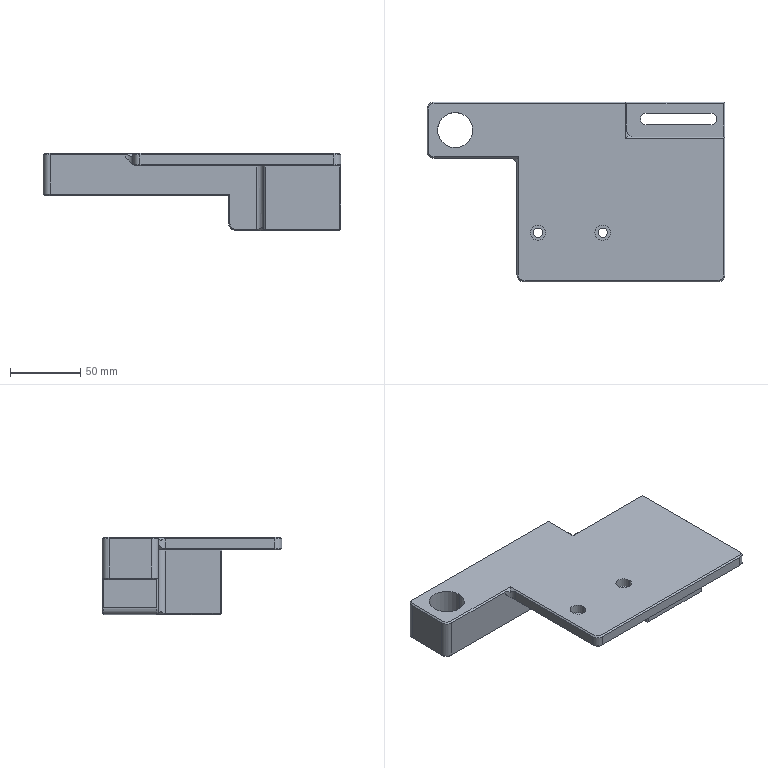NC program | NX | posted with a generic post | part box 212 x 128 x 55 mm
Lines 1 to 2819 of 8014, first 2439 of 2813 lines:
N10 G17 G21 G94 G90
(FLOOR_WALL_COPY_1 , TOOL : D50R0.8)
N12 T21 M6
N14 G54
N16 G17 G0 G90 X6.958 Y-91. S1200 M3
N18 G43 Z30. H21
N20 Z-0.45
N22 G94 G1 Y-63. F1200.
N24 X-101.
N26 G2 X-105. Y-59. R4.
N28 G1 Y-46.1
N30 X-41.603
N32 X-25.9 Y-30.397
N34 Y-1.1
N36 X41.
N38 Y-59.
N40 G2 X37. Y-63. R4.
N42 G1 X6.958
N44 Y-38.
N46 X-2.084
N48 G3 X-0.9 Y-30.397 R25.
N50 G1 Y-26.1
N52 X16.
N54 Y-38.
N56 X6.958
N58 Y-41.
N60 G0 Z30.
N62 Y-91.
N64 Z-0.9
N66 G1 Y-63.
N68 X-101.
N70 G2 X-105. Y-59. R4.
N72 G1 Y-46.1
N74 X-41.603
N76 X-25.9 Y-30.397
N78 Y-1.1
N80 X41.
N82 Y-59.
N84 G2 X37. Y-63. R4.
N86 G1 X6.958
N88 Y-38.
N90 X-2.084
N92 G3 X-0.9 Y-30.397 R25.
N94 G1 Y-26.1
N96 X16.
N98 Y-38.
N100 X6.958
N102 Y-41.
N104 G0 Z30.
N106 Y-91.
N108 Z-1.35
N110 G1 Y-63.
N112 X-101.
N114 G2 X-105. Y-59. R4.
N116 G1 Y-46.1
N118 X-41.603
N120 X-25.9 Y-30.397
N122 Y-1.1
N124 X41.
N126 Y-59.
N128 G2 X37. Y-63. R4.
N130 G1 X6.958
N132 Y-38.
N134 X-2.084
N136 G3 X-0.9 Y-30.397 R25.
N138 G1 Y-26.1
N140 X16.
N142 Y-38.
N144 X6.958
N146 Y-41.
N148 G0 Z30.
N150 Y-91.
N152 Z-1.8
N154 G1 Y-63.
N156 X-101.
N158 G2 X-105. Y-59. R4.
N160 G1 Y-46.1
N162 X-41.603
N164 X-25.9 Y-30.397
N166 Y-1.1
N168 X41.
N170 Y-59.
N172 G2 X37. Y-63. R4.
N174 G1 X6.958
N176 Y-38.
N178 X-2.084
N180 G3 X-0.9 Y-30.397 R25.
N182 G1 Y-26.1
N184 X16.
N186 Y-38.
N188 X6.958
N190 Y-41.
N192 G0 Z30.
N194 Y-91.
N196 Z-2.25
N198 G1 Y-63.
N200 X-101.
N202 G2 X-105. Y-59. R4.
N204 G1 Y-46.1
N206 X-41.603
N208 X-25.9 Y-30.397
N210 Y-1.1
N212 X41.
N214 Y-59.
N216 G2 X37. Y-63. R4.
N218 G1 X6.958
N220 Y-38.
N222 X-2.084
N224 G3 X-0.9 Y-30.397 R25.
N226 G1 Y-26.1
N228 X16.
N230 Y-38.
N232 X6.958
N234 Y-41.
N236 G0 Z30.
N238 Y-91.
N240 Z-2.7
N242 G1 Y-63.
N244 X-101.
N246 G2 X-105. Y-59. R4.
N248 G1 Y-46.1
N250 X-41.603
N252 X-25.9 Y-30.397
N254 Y-1.1
N256 X41.
N258 Y-59.
N260 G2 X37. Y-63. R4.
N262 G1 X6.958
N264 Y-38.
N266 X-2.084
N268 G3 X-0.9 Y-30.397 R25.
N270 G1 Y-26.1
N272 X16.
N274 Y-38.
N276 X6.958
N278 Y-41.
N280 G0 Z30.
N282 Y-91.
N284 Z-3.15
N286 G1 Y-63.
N288 X-101.
N290 G2 X-105. Y-59. R4.
N292 G1 Y-46.1
N294 X-41.603
N296 X-25.9 Y-30.397
N298 Y-1.1
N300 X41.
N302 Y-59.
N304 G2 X37. Y-63. R4.
N306 G1 X6.958
N308 Y-38.
N310 X-2.084
N312 G3 X-0.9 Y-30.397 R25.
N314 G1 Y-26.1
N316 X16.
N318 Y-38.
N320 X6.958
N322 Y-41.
N324 G0 Z30.
N326 Y-91.
N328 Z-3.6
N330 G1 Y-63.
N332 X-101.
N334 G2 X-105. Y-59. R4.
N336 G1 Y-46.1
N338 X-41.603
N340 X-25.9 Y-30.397
N342 Y-1.1
N344 X41.
N346 Y-59.
N348 G2 X37. Y-63. R4.
N350 G1 X6.958
N352 Y-38.
N354 X-2.084
N356 G3 X-0.9 Y-30.397 R25.
N358 G1 Y-26.1
N360 X16.
N362 Y-38.
N364 X6.958
N366 Y-41.
N368 G0 Z30.
N370 Y-91.
N372 Z-4.05
N374 G1 Y-63.
N376 X-101.
N378 G2 X-105. Y-59. R4.
N380 G1 Y-46.1
N382 X-41.603
N384 X-25.9 Y-30.397
N386 Y-1.1
N388 X41.
N390 Y-59.
N392 G2 X37. Y-63. R4.
N394 G1 X6.958
N396 Y-38.
N398 X-2.084
N400 G3 X-0.9 Y-30.397 R25.
N402 G1 Y-26.1
N404 X16.
N406 Y-38.
N408 X6.958
N410 Y-41.
N412 G0 Z30.
N414 Y-91.
N416 Z-4.5
N418 G1 Y-63.
N420 X-101.
N422 G2 X-105. Y-59. R4.
N424 G1 Y-46.1
N426 X-41.603
N428 X-25.9 Y-30.397
N430 Y-1.1
N432 X41.
N434 Y-59.
N436 G2 X37. Y-63. R4.
N438 G1 X6.958
N440 Y-38.
N442 X-2.084
N444 G3 X-0.9 Y-30.397 R25.
N446 G1 Y-26.1
N448 X16.
N450 Y-38.
N452 X6.958
N454 Y-41.
N456 G0 Z30.
N458 Y-91.
N460 Z-4.95
N462 G1 Y-63.
N464 X-101.
N466 G2 X-105. Y-59. R4.
N468 G1 Y-46.1
N470 X-41.603
N472 X-25.9 Y-30.397
N474 Y-1.1
N476 X41.
N478 Y-59.
N480 G2 X37. Y-63. R4.
N482 G1 X6.958
N484 Y-38.
N486 X-2.084
N488 G3 X-0.9 Y-30.397 R25.
N490 G1 Y-26.1
N492 X16.
N494 Y-38.
N496 X6.958
N498 Y-41.
N500 G0 Z30.
N502 Y-91.
N504 Z-5.4
N506 G1 Y-63.
N508 X-101.
N510 G2 X-105. Y-59. R4.
N512 G1 Y-46.1
N514 X-41.603
N516 X-25.9 Y-30.397
N518 Y-1.1
N520 X41.
N522 Y-59.
N524 G2 X37. Y-63. R4.
N526 G1 X6.958
N528 Y-38.
N530 X-2.084
N532 G3 X-0.9 Y-30.397 R25.
N534 G1 Y-26.1
N536 X16.
N538 Y-38.
N540 X6.958
N542 Y-41.
N544 G0 Z30.
N546 Y-91.
N548 Z-5.85
N550 G1 Y-63.
N552 X-101.
N554 G2 X-105. Y-59. R4.
N556 G1 Y-46.1
N558 X-41.603
N560 X-25.9 Y-30.397
N562 Y-1.1
N564 X41.
N566 Y-59.
N568 G2 X37. Y-63. R4.
N570 G1 X6.958
N572 Y-38.
N574 X-2.084
N576 G3 X-0.9 Y-30.397 R25.
N578 G1 Y-26.1
N580 X16.
N582 Y-38.
N584 X6.958
N586 Y-41.
N588 G0 Z30.
N590 Y-91.
N592 Z-6.3
N594 G1 Y-63.
N596 X-101.
N598 G2 X-105. Y-59. R4.
N600 G1 Y-46.1
N602 X-41.603
N604 X-25.9 Y-30.397
N606 Y-1.1
N608 X41.
N610 Y-59.
N612 G2 X37. Y-63. R4.
N614 G1 X6.958
N616 Y-38.
N618 X-2.084
N620 G3 X-0.9 Y-30.397 R25.
N622 G1 Y-26.1
N624 X16.
N626 Y-38.
N628 X6.958
N630 Y-41.
N632 G0 Z30.
N634 Y-91.
N636 Z-6.75
N638 G1 Y-63.
N640 X-101.
N642 G2 X-105. Y-59. R4.
N644 G1 Y-46.1
N646 X-41.603
N648 X-25.9 Y-30.397
N650 Y-1.1
N652 X41.
N654 Y-59.
N656 G2 X37. Y-63. R4.
N658 G1 X6.958
N660 Y-38.
N662 X-2.084
N664 G3 X-0.9 Y-30.397 R25.
N666 G1 Y-26.1
N668 X16.
N670 Y-38.
N672 X6.958
N674 Y-41.
N676 G0 Z30.
N678 Y-91.
N680 Z-7.2
N682 G1 Y-63.
N684 X-101.
N686 G2 X-105. Y-59. R4.
N688 G1 Y-46.1
N690 X-41.603
N692 X-25.9 Y-30.397
N694 Y-1.1
N696 X41.
N698 Y-59.
N700 G2 X37. Y-63. R4.
N702 G1 X6.958
N704 Y-38.
N706 X-2.084
N708 G3 X-0.9 Y-30.397 R25.
N710 G1 Y-26.1
N712 X16.
N714 Y-38.
N716 X6.958
N718 Y-41.
N720 G0 Z30.
N722 Y-91.
N724 Z-7.65
N726 G1 Y-63.
N728 X-101.
N730 G2 X-105. Y-59. R4.
N732 G1 Y-46.1
N734 X-41.603
N736 X-25.9 Y-30.397
N738 Y-1.1
N740 X41.
N742 Y-59.
N744 G2 X37. Y-63. R4.
N746 G1 X6.958
N748 Y-38.
N750 X-2.084
N752 G3 X-0.9 Y-30.397 R25.
N754 G1 Y-26.1
N756 X16.
N758 Y-38.
N760 X6.958
N762 Y-41.
N764 G0 Z30.
N766 Y-91.
N768 Z-8.1
N770 G1 Y-63.
N772 X-101.
N774 G2 X-105. Y-59. R4.
N776 G1 Y-46.1
N778 X-41.603
N780 X-25.9 Y-30.397
N782 Y-1.1
N784 X41.
N786 Y-59.
N788 G2 X37. Y-63. R4.
N790 G1 X6.958
N792 Y-38.
N794 X-2.084
N796 G3 X-0.9 Y-30.397 R25.
N798 G1 Y-26.1
N800 X16.
N802 Y-38.
N804 X6.958
N806 Y-41.
N808 G0 Z30.
N810 Y-91.
N812 Z-8.55
N814 G1 Y-63.
N816 X-101.
N818 G2 X-105. Y-59. R4.
N820 G1 Y-46.1
N822 X-41.603
N824 X-25.9 Y-30.397
N826 Y-1.1
N828 X41.
N830 Y-59.
N832 G2 X37. Y-63. R4.
N834 G1 X6.958
N836 Y-38.
N838 X-2.084
N840 G3 X-0.9 Y-30.397 R25.
N842 G1 Y-26.1
N844 X16.
N846 Y-38.
N848 X6.958
N850 Y-41.
N852 G0 Z30.
N854 Y-91.
N856 Z-9.
N858 G1 Y-63.
N860 X-101.
N862 G2 X-105. Y-59. R4.
N864 G1 Y-46.1
N866 X-41.603
N868 X-25.9 Y-30.397
N870 Y-1.1
N872 X41.
N874 Y-59.
N876 G2 X37. Y-63. R4.
N878 G1 X6.958
N880 Y-38.
N882 X-2.084
N884 G3 X-0.9 Y-30.397 R25.
N886 G1 Y-26.1
N888 X16.
N890 Y-38.
N892 X6.958
N894 Y-41.
N896 G0 Z30.
N898 Y-91.
N900 Z-9.45
N902 G1 Y-63.
N904 X-101.
N906 G2 X-105. Y-59. R4.
N908 G1 Y-46.1
N910 X-41.603
N912 X-25.9 Y-30.397
N914 Y-1.1
N916 X41.
N918 Y-59.
N920 G2 X37. Y-63. R4.
N922 G1 X6.958
N924 Y-38.
N926 X-2.084
N928 G3 X-0.9 Y-30.397 R25.
N930 G1 Y-26.1
N932 X16.
N934 Y-38.
N936 X6.958
N938 Y-41.
N940 G0 Z30.
N942 Y-91.
N944 Z-9.9
N946 G1 Y-63.
N948 X-101.
N950 G2 X-105. Y-59. R4.
N952 G1 Y-46.1
N954 X-41.603
N956 X-25.9 Y-30.397
N958 Y-1.1
N960 X41.
N962 Y-59.
N964 G2 X37. Y-63. R4.
N966 G1 X6.958
N968 Y-38.
N970 X-2.084
N972 G3 X-0.9 Y-30.397 R25.
N974 G1 Y-26.1
N976 X16.
N978 Y-38.
N980 X6.958
N982 Y-41.
N984 G0 Z30.
N986 Y-91.
N988 Z-10.35
N990 G1 Y-63.
N992 X-101.
N994 G2 X-105. Y-59. R4.
N996 G1 Y-46.1
N998 X-41.603
N1000 X-25.9 Y-30.397
N1002 Y-1.1
N1004 X41.
N1006 Y-59.
N1008 G2 X37. Y-63. R4.
N1010 G1 X6.958
N1012 Y-38.
N1014 X-2.084
N1016 G3 X-0.9 Y-30.397 R25.
N1018 G1 Y-26.1
N1020 X16.
N1022 Y-38.
N1024 X6.958
N1026 Y-41.
N1028 G0 Z30.
N1030 Y-91.
N1032 Z-10.8
N1034 G1 Y-63.
N1036 X-101.
N1038 G2 X-105. Y-59. R4.
N1040 G1 Y-46.1
N1042 X-41.603
N1044 X-25.9 Y-30.397
N1046 Y-1.1
N1048 X41.
N1050 Y-59.
N1052 G2 X37. Y-63. R4.
N1054 G1 X6.958
N1056 Y-38.
N1058 X-2.084
N1060 G3 X-0.9 Y-30.397 R25.
N1062 G1 Y-26.1
N1064 X16.
N1066 Y-38.
N1068 X6.958
N1070 Y-41.
N1072 G0 Z30.
N1074 Y-91.
N1076 Z-11.25
N1078 G1 Y-63.
N1080 X-101.
N1082 G2 X-105. Y-59. R4.
N1084 G1 Y-46.1
N1086 X-41.603
N1088 X-25.9 Y-30.397
N1090 Y-1.1
N1092 X41.
N1094 Y-59.
N1096 G2 X37. Y-63. R4.
N1098 G1 X6.958
N1100 Y-38.
N1102 X-2.084
N1104 G3 X-0.9 Y-30.397 R25.
N1106 G1 Y-26.1
N1108 X16.
N1110 Y-38.
N1112 X6.958
N1114 Y-41.
N1116 G0 Z30.
N1118 Y-91.
N1120 Z-11.7
N1122 G1 Y-63.
N1124 X-101.
N1126 G2 X-105. Y-59. R4.
N1128 G1 Y-46.1
N1130 X-41.603
N1132 X-25.9 Y-30.397
N1134 Y-1.1
N1136 X41.
N1138 Y-59.
N1140 G2 X37. Y-63. R4.
N1142 G1 X6.958
N1144 Y-38.
N1146 X-2.084
N1148 G3 X-0.9 Y-30.397 R25.
N1150 G1 Y-26.1
N1152 X16.
N1154 Y-38.
N1156 X6.958
N1158 Y-41.
N1160 G0 Z30.
N1162 Y-91.
N1164 Z-12.15
N1166 G1 Y-63.
N1168 X-101.
N1170 G2 X-105. Y-59. R4.
N1172 G1 Y-46.1
N1174 X-41.603
N1176 X-25.9 Y-30.397
N1178 Y-1.1
N1180 X41.
N1182 Y-59.
N1184 G2 X37. Y-63. R4.
N1186 G1 X6.958
N1188 Y-38.
N1190 X-2.084
N1192 G3 X-0.9 Y-30.397 R25.
N1194 G1 Y-26.1
N1196 X16.
N1198 Y-38.
N1200 X6.958
N1202 Y-41.
N1204 G0 Z30.
N1206 Y-91.
N1208 Z-12.6
N1210 G1 Y-63.
N1212 X-101.
N1214 G2 X-105. Y-59. R4.
N1216 G1 Y-46.1
N1218 X-41.603
N1220 X-25.9 Y-30.397
N1222 Y-1.1
N1224 X41.
N1226 Y-59.
N1228 G2 X37. Y-63. R4.
N1230 G1 X6.958
N1232 Y-38.
N1234 X-2.084
N1236 G3 X-0.9 Y-30.397 R25.
N1238 G1 Y-26.1
N1240 X16.
N1242 Y-38.
N1244 X6.958
N1246 Y-41.
N1248 G0 Z30.
N1250 Y-91.
N1252 Z-13.05
N1254 G1 Y-63.
N1256 X-101.
N1258 G2 X-105. Y-59. R4.
N1260 G1 Y-46.1
N1262 X-41.603
N1264 X-25.9 Y-30.397
N1266 Y-1.1
N1268 X41.
N1270 Y-59.
N1272 G2 X37. Y-63. R4.
N1274 G1 X6.958
N1276 Y-38.
N1278 X-2.084
N1280 G3 X-0.9 Y-30.397 R25.
N1282 G1 Y-26.1
N1284 X16.
N1286 Y-38.
N1288 X6.958
N1290 Y-41.
N1292 G0 Z30.
N1294 Y-91.
N1296 Z-13.5
N1298 G1 Y-63.
N1300 X-101.
N1302 G2 X-105. Y-59. R4.
N1304 G1 Y-46.1
N1306 X-41.603
N1308 X-25.9 Y-30.397
N1310 Y-1.1
N1312 X41.
N1314 Y-59.
N1316 G2 X37. Y-63. R4.
N1318 G1 X6.958
N1320 Y-38.
N1322 X-2.084
N1324 G3 X-0.9 Y-30.397 R25.
N1326 G1 Y-26.1
N1328 X16.
N1330 Y-38.
N1332 X6.958
N1334 Y-41.
N1336 G0 Z30.
N1338 Y-91.
N1340 Z-13.95
N1342 G1 Y-63.
N1344 X-101.
N1346 G2 X-105. Y-59. R4.
N1348 G1 Y-46.1
N1350 X-41.603
N1352 X-25.9 Y-30.397
N1354 Y-1.1
N1356 X41.
N1358 Y-59.
N1360 G2 X37. Y-63. R4.
N1362 G1 X6.958
N1364 Y-38.
N1366 X-2.084
N1368 G3 X-0.9 Y-30.397 R25.
N1370 G1 Y-26.1
N1372 X16.
N1374 Y-38.
N1376 X6.958
N1378 Y-41.
N1380 G0 Z30.
N1382 Y-91.
N1384 Z-14.4
N1386 G1 Y-63.
N1388 X-101.
N1390 G2 X-105. Y-59. R4.
N1392 G1 Y-46.1
N1394 X-41.603
N1396 X-25.9 Y-30.397
N1398 Y-1.1
N1400 X41.
N1402 Y-59.
N1404 G2 X37. Y-63. R4.
N1406 G1 X6.958
N1408 Y-38.
N1410 X-2.084
N1412 G3 X-0.9 Y-30.397 R25.
N1414 G1 Y-26.1
N1416 X16.
N1418 Y-38.
N1420 X6.958
N1422 Y-41.
N1424 G0 Z30.
N1426 Y-91.
N1428 Z-14.85
N1430 G1 Y-63.
N1432 X-101.
N1434 G2 X-105. Y-59. R4.
N1436 G1 Y-46.1
N1438 X-41.603
N1440 X-25.9 Y-30.397
N1442 Y-1.1
N1444 X41.
N1446 Y-59.
N1448 G2 X37. Y-63. R4.
N1450 G1 X6.958
N1452 Y-38.
N1454 X-2.084
N1456 G3 X-0.9 Y-30.397 R25.
N1458 G1 Y-26.1
N1460 X16.
N1462 Y-38.
N1464 X6.958
N1466 Y-41.
N1468 G0 Z30.
N1470 Y-91.
N1472 Z-15.3
N1474 G1 Y-63.
N1476 X-101.
N1478 G2 X-105. Y-59. R4.
N1480 G1 Y-46.1
N1482 X-41.603
N1484 X-25.9 Y-30.397
N1486 Y-1.1
N1488 X41.
N1490 Y-59.
N1492 G2 X37. Y-63. R4.
N1494 G1 X6.958
N1496 Y-38.
N1498 X-2.084
N1500 G3 X-0.9 Y-30.397 R25.
N1502 G1 Y-26.1
N1504 X16.
N1506 Y-38.
N1508 X6.958
N1510 Y-41.
N1512 G0 Z30.
N1514 Y-91.
N1516 Z-15.75
N1518 G1 Y-63.
N1520 X-101.
N1522 G2 X-105. Y-59. R4.
N1524 G1 Y-46.1
N1526 X-41.603
N1528 X-25.9 Y-30.397
N1530 Y-1.1
N1532 X41.
N1534 Y-59.
N1536 G2 X37. Y-63. R4.
N1538 G1 X6.958
N1540 Y-38.
N1542 X-2.084
N1544 G3 X-0.9 Y-30.397 R25.
N1546 G1 Y-26.1
N1548 X16.
N1550 Y-38.
N1552 X6.958
N1554 Y-41.
N1556 G0 Z30.
N1558 Y-91.
N1560 Z-16.2
N1562 G1 Y-63.
N1564 X-101.
N1566 G2 X-105. Y-59. R4.
N1568 G1 Y-46.1
N1570 X-41.603
N1572 X-25.9 Y-30.397
N1574 Y-1.1
N1576 X41.
N1578 Y-59.
N1580 G2 X37. Y-63. R4.
N1582 G1 X6.958
N1584 Y-38.
N1586 X-2.084
N1588 G3 X-0.9 Y-30.397 R25.
N1590 G1 Y-26.1
N1592 X16.
N1594 Y-38.
N1596 X6.958
N1598 Y-41.
N1600 G0 Z30.
N1602 Y-91.
N1604 Z-16.65
N1606 G1 Y-63.
N1608 X-101.
N1610 G2 X-105. Y-59. R4.
N1612 G1 Y-46.1
N1614 X-41.603
N1616 X-25.9 Y-30.397
N1618 Y-1.1
N1620 X41.
N1622 Y-59.
N1624 G2 X37. Y-63. R4.
N1626 G1 X6.958
N1628 Y-38.
N1630 X-2.084
N1632 G3 X-0.9 Y-30.397 R25.
N1634 G1 Y-26.1
N1636 X16.
N1638 Y-38.
N1640 X6.958
N1642 Y-41.
N1644 G0 Z30.
N1646 Y-91.
N1648 Z-17.1
N1650 G1 Y-63.
N1652 X-101.
N1654 G2 X-105. Y-59. R4.
N1656 G1 Y-46.1
N1658 X-41.603
N1660 X-25.9 Y-30.397
N1662 Y-1.1
N1664 X41.
N1666 Y-59.
N1668 G2 X37. Y-63. R4.
N1670 G1 X6.958
N1672 Y-38.
N1674 X-2.084
N1676 G3 X-0.9 Y-30.397 R25.
N1678 G1 Y-26.1
N1680 X16.
N1682 Y-38.
N1684 X6.958
N1686 Y-41.
N1688 G0 Z30.
N1690 Y-91.
N1692 Z-17.55
N1694 G1 Y-63.
N1696 X-101.
N1698 G2 X-105. Y-59. R4.
N1700 G1 Y-46.1
N1702 X-41.603
N1704 X-25.9 Y-30.397
N1706 Y-1.1
N1708 X41.
N1710 Y-59.
N1712 G2 X37. Y-63. R4.
N1714 G1 X6.958
N1716 Y-38.
N1718 X-2.084
N1720 G3 X-0.9 Y-30.397 R25.
N1722 G1 Y-26.1
N1724 X16.
N1726 Y-38.
N1728 X6.958
N1730 Y-41.
N1732 G0 Z30.
N1734 Y-91.
N1736 Z-18.
N1738 G1 Y-63.
N1740 X-101.
N1742 G2 X-105. Y-59. R4.
N1744 G1 Y-46.1
N1746 X-41.603
N1748 X-25.9 Y-30.397
N1750 Y-1.1
N1752 X41.
N1754 Y-59.
N1756 G2 X37. Y-63. R4.
N1758 G1 X6.958
N1760 Y-38.
N1762 X-2.084
N1764 G3 X-0.9 Y-30.397 R25.
N1766 G1 Y-26.1
N1768 X16.
N1770 Y-38.
N1772 X6.958
N1774 Y-41.
N1776 G0 Z30.
N1778 Y-91.
N1780 Z-18.45
N1782 G1 Y-63.
N1784 X-101.
N1786 G2 X-105. Y-59. R4.
N1788 G1 Y-46.1
N1790 X-41.603
N1792 X-25.9 Y-30.397
N1794 Y-1.1
N1796 X41.
N1798 Y-59.
N1800 G2 X37. Y-63. R4.
N1802 G1 X6.958
N1804 Y-38.
N1806 X-2.084
N1808 G3 X-0.9 Y-30.397 R25.
N1810 G1 Y-26.1
N1812 X16.
N1814 Y-38.
N1816 X6.958
N1818 Y-41.
N1820 G0 Z30.
N1822 Y-91.
N1824 Z-18.9
N1826 G1 Y-63.
N1828 X-101.
N1830 G2 X-105. Y-59. R4.
N1832 G1 Y-46.1
N1834 X-41.603
N1836 X-25.9 Y-30.397
N1838 Y-1.1
N1840 X41.
N1842 Y-59.
N1844 G2 X37. Y-63. R4.
N1846 G1 X6.958
N1848 Y-38.
N1850 X-2.084
N1852 G3 X-0.9 Y-30.397 R25.
N1854 G1 Y-26.1
N1856 X16.
N1858 Y-38.
N1860 X6.958
N1862 Y-41.
N1864 G0 Z30.
N1866 Y-91.
N1868 Z-19.35
N1870 G1 Y-63.
N1872 X-101.
N1874 G2 X-105. Y-59. R4.
N1876 G1 Y-46.1
N1878 X-41.603
N1880 X-25.9 Y-30.397
N1882 Y-1.1
N1884 X41.
N1886 Y-59.
N1888 G2 X37. Y-63. R4.
N1890 G1 X6.958
N1892 Y-38.
N1894 X-2.084
N1896 G3 X-0.9 Y-30.397 R25.
N1898 G1 Y-26.1
N1900 X16.
N1902 Y-38.
N1904 X6.958
N1906 Y-41.
N1908 G0 Z30.
N1910 Y-91.
N1912 Z-19.8
N1914 G1 Y-63.
N1916 X-101.
N1918 G2 X-105. Y-59. R4.
N1920 G1 Y-46.1
N1922 X-41.603
N1924 X-25.9 Y-30.397
N1926 Y-1.1
N1928 X41.
N1930 Y-59.
N1932 G2 X37. Y-63. R4.
N1934 G1 X6.958
N1936 Y-38.
N1938 X-2.084
N1940 G3 X-0.9 Y-30.397 R25.
N1942 G1 Y-26.1
N1944 X16.
N1946 Y-38.
N1948 X6.958
N1950 Y-41.
N1952 G0 Z30.
N1954 Y-91.
N1956 Z-20.25
N1958 G1 Y-63.
N1960 X-101.
N1962 G2 X-105. Y-59. R4.
N1964 G1 Y-46.1
N1966 X-41.603
N1968 X-25.9 Y-30.397
N1970 Y-1.1
N1972 X41.
N1974 Y-59.
N1976 G2 X37. Y-63. R4.
N1978 G1 X6.958
N1980 Y-38.
N1982 X-2.084
N1984 G3 X-0.9 Y-30.397 R25.
N1986 G1 Y-26.1
N1988 X16.
N1990 Y-38.
N1992 X6.958
N1994 Y-41.
N1996 G0 Z30.
N1998 Y-91.
N2000 Z-20.7
N2002 G1 Y-63.
N2004 X-101.
N2006 G2 X-105. Y-59. R4.
N2008 G1 Y-46.1
N2010 X-41.603
N2012 X-25.9 Y-30.397
N2014 Y-1.1
N2016 X41.
N2018 Y-59.
N2020 G2 X37. Y-63. R4.
N2022 G1 X6.958
N2024 Y-38.
N2026 X-2.084
N2028 G3 X-0.9 Y-30.397 R25.
N2030 G1 Y-26.1
N2032 X16.
N2034 Y-38.
N2036 X6.958
N2038 Y-41.
N2040 G0 Z30.
N2042 Y-91.
N2044 Z-21.15
N2046 G1 Y-63.
N2048 X-101.
N2050 G2 X-105. Y-59. R4.
N2052 G1 Y-46.1
N2054 X-41.603
N2056 X-25.9 Y-30.397
N2058 Y-1.1
N2060 X41.
N2062 Y-59.
N2064 G2 X37. Y-63. R4.
N2066 G1 X6.958
N2068 Y-38.
N2070 X-2.084
N2072 G3 X-0.9 Y-30.397 R25.
N2074 G1 Y-26.1
N2076 X16.
N2078 Y-38.
N2080 X6.958
N2082 Y-41.
N2084 G0 Z30.
N2086 Y-91.
N2088 Z-21.6
N2090 G1 Y-63.
N2092 X-101.
N2094 G2 X-105. Y-59. R4.
N2096 G1 Y-46.1
N2098 X-41.603
N2100 X-25.9 Y-30.397
N2102 Y-1.1
N2104 X41.
N2106 Y-59.
N2108 G2 X37. Y-63. R4.
N2110 G1 X6.958
N2112 Y-38.
N2114 X-2.084
N2116 G3 X-0.9 Y-30.397 R25.
N2118 G1 Y-26.1
N2120 X16.
N2122 Y-38.
N2124 X6.958
N2126 Y-41.
N2128 G0 Z30.
N2130 Y-91.
N2132 Z-22.05
N2134 G1 Y-63.
N2136 X-101.
N2138 G2 X-105. Y-59. R4.
N2140 G1 Y-46.1
N2142 X-41.603
N2144 X-25.9 Y-30.397
N2146 Y-1.1
N2148 X41.
N2150 Y-59.
N2152 G2 X37. Y-63. R4.
N2154 G1 X6.958
N2156 Y-38.
N2158 X-2.084
N2160 G3 X-0.9 Y-30.397 R25.
N2162 G1 Y-26.1
N2164 X16.
N2166 Y-38.
N2168 X6.958
N2170 Y-41.
N2172 G0 Z30.
N2174 Y-91.
N2176 Z-22.5
N2178 G1 Y-63.
N2180 X-101.
N2182 G2 X-105. Y-59. R4.
N2184 G1 Y-46.1
N2186 X-41.603
N2188 X-25.9 Y-30.397
N2190 Y-1.1
N2192 X41.
N2194 Y-59.
N2196 G2 X37. Y-63. R4.
N2198 G1 X6.958
N2200 Y-38.
N2202 X-2.084
N2204 G3 X-0.9 Y-30.397 R25.
N2206 G1 Y-26.1
N2208 X16.
N2210 Y-38.
N2212 X6.958
N2214 Y-41.
N2216 G0 Z30.
N2218 Y-91.
N2220 Z-22.95
N2222 G1 Y-63.
N2224 X-101.
N2226 G2 X-105. Y-59. R4.
N2228 G1 Y-46.1
N2230 X-41.603
N2232 X-25.9 Y-30.397
N2234 Y-1.1
N2236 X41.
N2238 Y-59.
N2240 G2 X37. Y-63. R4.
N2242 G1 X6.958
N2244 Y-38.
N2246 X-2.084
N2248 G3 X-0.9 Y-30.397 R25.
N2250 G1 Y-26.1
N2252 X16.
N2254 Y-38.
N2256 X6.958
N2258 Y-41.
N2260 G0 Z30.
N2262 Y-91.
N2264 Z-23.4
N2266 G1 Y-63.
N2268 X-101.
N2270 G2 X-105. Y-59. R4.
N2272 G1 Y-46.1
N2274 X-41.603
N2276 X-25.9 Y-30.397
N2278 Y-1.1
N2280 X41.
N2282 Y-59.
N2284 G2 X37. Y-63. R4.
N2286 G1 X6.958
N2288 Y-38.
N2290 X-2.084
N2292 G3 X-0.9 Y-30.397 R25.
N2294 G1 Y-26.1
N2296 X16.
N2298 Y-38.
N2300 X6.958
N2302 Y-41.
N2304 G0 Z30.
N2306 Y-91.
N2308 Z-23.85
N2310 G1 Y-63.
N2312 X-101.
N2314 G2 X-105. Y-59. R4.
N2316 G1 Y-46.1
N2318 X-41.603
N2320 X-25.9 Y-30.397
N2322 Y-1.1
N2324 X41.
N2326 Y-59.
N2328 G2 X37. Y-63. R4.
N2330 G1 X6.958
N2332 Y-38.
N2334 X-2.084
N2336 G3 X-0.9 Y-30.397 R25.
N2338 G1 Y-26.1
N2340 X16.
N2342 Y-38.
N2344 X6.958
N2346 Y-41.
N2348 G0 Z30.
N2350 Y-91.
N2352 Z-24.3
N2354 G1 Y-63.
N2356 X-101.
N2358 G2 X-105. Y-59. R4.
N2360 G1 Y-46.1
N2362 X-41.603
N2364 X-25.9 Y-30.397
N2366 Y-1.1
N2368 X41.
N2370 Y-59.
N2372 G2 X37. Y-63. R4.
N2374 G1 X6.958
N2376 Y-38.
N2378 X-2.084
N2380 G3 X-0.9 Y-30.397 R25.
N2382 G1 Y-26.1
N2384 X16.
N2386 Y-38.
N2388 X6.958
N2390 Y-41.
N2392 G0 Z30.
N2394 Y-91.
N2396 Z-24.75
N2398 G1 Y-63.
N2400 X-101.
N2402 G2 X-105. Y-59. R4.
N2404 G1 Y-46.1
N2406 X-41.603
N2408 X-25.9 Y-30.397
N2410 Y-1.1
N2412 X41.
N2414 Y-59.
N2416 G2 X37. Y-63. R4.
N2418 G1 X6.958
N2420 Y-38.
N2422 X-2.084
N2424 G3 X-0.9 Y-30.397 R25.
N2426 G1 Y-26.1
N2428 X16.
N2430 Y-38.
N2432 X6.958
N2434 Y-41.
N2436 G0 Z30.
N2438 Y-91.
N2440 Z-25.2
N2442 G1 Y-63.
N2444 X-101.
N2446 G2 X-105. Y-59. R4.
N2448 G1 Y-46.1
N2450 X-41.603
N2452 X-25.9 Y-30.397
N2454 Y-1.1
N2456 X41.
N2458 Y-59.
N2460 G2 X37. Y-63. R4.
N2462 G1 X6.958
N2464 Y-38.
N2466 X-2.084
N2468 G3 X-0.9 Y-30.397 R25.
N2470 G1 Y-26.1
N2472 X16.
N2474 Y-38.
N2476 X6.958
N2478 Y-41.
N2480 G0 Z30.
N2482 Y-91.
N2484 Z-25.65
N2486 G1 Y-63.
N2488 X-101.
N2490 G2 X-105. Y-59. R4.
N2492 G1 Y-46.1
N2494 X-41.603
N2496 X-25.9 Y-30.397
N2498 Y-1.1
N2500 X41.
N2502 Y-59.
N2504 G2 X37. Y-63. R4.
N2506 G1 X6.958
N2508 Y-38.
N2510 X-2.084
N2512 G3 X-0.9 Y-30.397 R25.
N2514 G1 Y-26.1
N2516 X16.
N2518 Y-38.
N2520 X6.958
N2522 Y-41.
N2524 G0 Z30.
N2526 Y-91.
N2528 Z-26.1
N2530 G1 Y-63.
N2532 X-101.
N2534 G2 X-105. Y-59. R4.
N2536 G1 Y-46.1
N2538 X-41.603
N2540 X-25.9 Y-30.397
N2542 Y-1.1
N2544 X41.
N2546 Y-59.
N2548 G2 X37. Y-63. R4.
N2550 G1 X6.958
N2552 Y-38.
N2554 X-2.084
N2556 G3 X-0.9 Y-30.397 R25.
N2558 G1 Y-26.1
N2560 X16.
N2562 Y-38.
N2564 X6.958
N2566 Y-41.
N2568 G0 Z30.
N2570 Y-91.
N2572 Z-26.55
N2574 G1 Y-63.
N2576 X-101.
N2578 G2 X-105. Y-59. R4.
N2580 G1 Y-46.1
N2582 X-41.603
N2584 X-25.9 Y-30.397
N2586 Y-1.1
N2588 X41.
N2590 Y-59.
N2592 G2 X37. Y-63. R4.
N2594 G1 X6.958
N2596 Y-38.
N2598 X-2.084
N2600 G3 X-0.9 Y-30.397 R25.
N2602 G1 Y-26.1
N2604 X16.
N2606 Y-38.
N2608 X6.958
N2610 Y-41.
N2612 G0 Z30.
N2614 Y-91.
N2616 Z-27.
N2618 G1 Y-63.
N2620 X-101.
N2622 G2 X-105. Y-59. R4.
N2624 G1 Y-46.1
N2626 X-41.603
N2628 X-25.9 Y-30.397
N2630 Y-1.1
N2632 X41.
N2634 Y-59.
N2636 G2 X37. Y-63. R4.
N2638 G1 X6.958
N2640 Y-38.
N2642 X-2.084
N2644 G3 X-0.9 Y-30.397 R25.
N2646 G1 Y-26.1
N2648 X16.
N2650 Y-38.
N2652 X6.958
N2654 Y-41.
N2656 G0 Z30.
N2658 Y-91.
N2660 Z-27.45
N2662 G1 Y-63.
N2664 X-101.
N2666 G2 X-105. Y-59. R4.
N2668 G1 Y-46.1
N2670 X-41.603
N2672 X-25.9 Y-30.397
N2674 Y-1.1
N2676 X41.
N2678 Y-59.
N2680 G2 X37. Y-63. R4.
N2682 G1 X6.958
N2684 Y-38.
N2686 X-2.084
N2688 G3 X-0.9 Y-30.397 R25.
N2690 G1 Y-26.1
N2692 X16.
N2694 Y-38.
N2696 X6.958
N2698 Y-41.
N2700 G0 Z30.
N2702 Y-91.
N2704 Z-27.9
N2706 G1 Y-63.
N2708 X-101.
N2710 G2 X-105. Y-59. R4.
N2712 G1 Y-46.1
N2714 X-41.603
N2716 X-25.9 Y-30.397
N2718 Y-1.1
N2720 X41.
N2722 Y-59.
N2724 G2 X37. Y-63. R4.
N2726 G1 X6.958
N2728 Y-38.
N2730 X-2.084
N2732 G3 X-0.9 Y-30.397 R25.
N2734 G1 Y-26.1
N2736 X16.
N2738 Y-38.
N2740 X6.958
N2742 Y-41.
N2744 G0 Z30.
N2746 Y-91.
N2748 Z-28.35
N2750 G1 Y-63.
N2752 X-101.
N2754 G2 X-105. Y-59. R4.
N2756 G1 Y-46.1
N2758 X-41.603
N2760 X-25.9 Y-30.397
N2762 Y-1.1
N2764 X41.
N2766 Y-59.
N2768 G2 X37. Y-63. R4.
N2770 G1 X6.958
N2772 Y-38.
N2774 X-2.084
N2776 G3 X-0.9 Y-30.397 R25.
N2778 G1 Y-26.1
N2780 X16.
N2782 Y-38.
N2784 X6.958
N2786 Y-41.
N2788 G0 Z30.
N2790 Y-91.
N2792 Z-28.8
N2794 G1 Y-63.
N2796 X-101.
N2798 G2 X-105. Y-59. R4.
N2800 G1 Y-46.1
N2802 X-41.603
N2804 X-25.9 Y-30.397
N2806 Y-1.1
N2808 X41.
N2810 Y-59.
N2812 G2 X37. Y-63. R4.
N2814 G1 X6.958
N2816 Y-38.
N2818 X-2.084
N2820 G3 X-0.9 Y-30.397 R25.
N2822 G1 Y-26.1
N2824 X16.
N2826 Y-38.
N2828 X6.958
N2830 Y-41.
N2832 G0 Z30.
N2834 Y-91.
N2836 Z-29.25
N2838 G1 Y-63.
N2840 X-101.
N2842 G2 X-105. Y-59. R4.
N2844 G1 Y-46.1
N2846 X-41.603
N2848 X-25.9 Y-30.397
N2850 Y-1.1
N2852 X41.
N2854 Y-59.
N2856 G2 X37. Y-63. R4.
N2858 G1 X6.958
N2860 Y-38.
N2862 X-2.084
N2864 G3 X-0.9 Y-30.397 R25.
N2866 G1 Y-26.1
N2868 X16.
N2870 Y-38.
N2872 X6.958
N2874 Y-41.
N2876 G0 Z30.
N2878 Y-91.
N2880 Z-29.7
N2882 G1 Y-63.
N2884 X-101.
N2886 G2 X-105. Y-59. R4.
N2888 G1 Y-46.1
N2890 X-41.603
N2892 X-25.9 Y-30.397
N2894 Y-1.1
N2896 X41.
N2898 Y-59.
N2900 G2 X37. Y-63. R4.
N2902 G1 X6.958
N2904 Y-38.
N2906 X-2.084
N2908 G3 X-0.9 Y-30.397 R25.
N2910 G1 Y-26.1
N2912 X16.
N2914 Y-38.
N2916 X6.958
N2918 Y-41.
N2920 G0 Z30.
N2922 Y-91.
N2924 Z-30.15
N2926 G1 Y-63.
N2928 X-101.
N2930 G2 X-105. Y-59. R4.
N2932 G1 Y-46.1
N2934 X-41.603
N2936 X-25.9 Y-30.397
N2938 Y-1.1
N2940 X41.
N2942 Y-59.
N2944 G2 X37. Y-63. R4.
N2946 G1 X6.958
N2948 Y-38.
N2950 X-2.084
N2952 G3 X-0.9 Y-30.397 R25.
N2954 G1 Y-26.1
N2956 X16.
N2958 Y-38.
N2960 X6.958
N2962 Y-41.
N2964 G0 Z30.
N2966 Y-91.
N2968 Z-30.6
N2970 G1 Y-63.
N2972 X-101.
N2974 G2 X-105. Y-59. R4.
N2976 G1 Y-46.1
N2978 X-41.603
N2980 X-25.9 Y-30.397
N2982 Y-1.1
N2984 X41.
N2986 Y-59.
N2988 G2 X37. Y-63. R4.
N2990 G1 X6.958
N2992 Y-38.
N2994 X-2.084
N2996 G3 X-0.9 Y-30.397 R25.
N2998 G1 Y-26.1
N3000 X16.
N3002 Y-38.
N3004 X6.958
N3006 Y-41.
N3008 G0 Z30.
N3010 Y-91.
N3012 Z-31.05
N3014 G1 Y-63.
N3016 X-101.
N3018 G2 X-105. Y-59. R4.
N3020 G1 Y-46.1
N3022 X-41.603
N3024 X-25.9 Y-30.397
N3026 Y-1.1
N3028 X41.
N3030 Y-59.
N3032 G2 X37. Y-63. R4.
N3034 G1 X6.958
N3036 Y-38.
N3038 X-2.084
N3040 G3 X-0.9 Y-30.397 R25.
N3042 G1 Y-26.1
N3044 X16.
N3046 Y-38.
N3048 X6.958
N3050 Y-41.
N3052 G0 Z30.
N3054 Y-91.
N3056 Z-31.5
N3058 G1 Y-63.
N3060 X-101.
N3062 G2 X-105. Y-59. R4.
N3064 G1 Y-46.1
N3066 X-41.603
N3068 X-25.9 Y-30.397
N3070 Y-1.1
N3072 X41.
N3074 Y-59.
N3076 G2 X37. Y-63. R4.
N3078 G1 X6.958
N3080 Y-38.
N3082 X-2.084
N3084 G3 X-0.9 Y-30.397 R25.
N3086 G1 Y-26.1
N3088 X16.
N3090 Y-38.
N3092 X6.958
N3094 Y-41.
N3096 G0 Z30.
N3098 Y-91.
N3100 Z-31.95
N3102 G1 Y-63.
N3104 X-101.
N3106 G2 X-105. Y-59. R4.
N3108 G1 Y-46.1
N3110 X-41.603
N3112 X-25.9 Y-30.397
N3114 Y-1.1
N3116 X41.
N3118 Y-59.
N3120 G2 X37. Y-63. R4.
N3122 G1 X6.958
N3124 Y-38.
N3126 X-2.084
N3128 G3 X-0.9 Y-30.397 R25.
N3130 G1 Y-26.1
N3132 X16.
N3134 Y-38.
N3136 X6.958
N3138 Y-41.
N3140 G0 Z30.
N3142 Y-91.
N3144 Z-32.4
N3146 G1 Y-63.
N3148 X-101.
N3150 G2 X-105. Y-59. R4.
N3152 G1 Y-46.1
N3154 X-41.603
N3156 X-25.9 Y-30.397
N3158 Y-1.1
N3160 X41.
N3162 Y-59.
N3164 G2 X37. Y-63. R4.
N3166 G1 X6.958
N3168 Y-38.
N3170 X-2.084
N3172 G3 X-0.9 Y-30.397 R25.
N3174 G1 Y-26.1
N3176 X16.
N3178 Y-38.
N3180 X6.958
N3182 Y-41.
N3184 G0 Z30.
N3186 Y-91.
N3188 Z-32.85
N3190 G1 Y-63.
N3192 X-101.
N3194 G2 X-105. Y-59. R4.
N3196 G1 Y-46.1
N3198 X-41.603
N3200 X-25.9 Y-30.397
N3202 Y-1.1
N3204 X41.
N3206 Y-59.
N3208 G2 X37. Y-63. R4.
N3210 G1 X6.958
N3212 Y-38.
N3214 X-2.084
N3216 G3 X-0.9 Y-30.397 R25.
N3218 G1 Y-26.1
N3220 X16.
N3222 Y-38.
N3224 X6.958
N3226 Y-41.
N3228 G0 Z30.
N3230 Y-91.
N3232 Z-33.3
N3234 G1 Y-63.
N3236 X-101.
N3238 G2 X-105. Y-59. R4.
N3240 G1 Y-46.1
N3242 X-41.603
N3244 X-25.9 Y-30.397
N3246 Y-1.1
N3248 X41.
N3250 Y-59.
N3252 G2 X37. Y-63. R4.
N3254 G1 X6.958
N3256 Y-38.
N3258 X-2.084
N3260 G3 X-0.9 Y-30.397 R25.
N3262 G1 Y-26.1
N3264 X16.
N3266 Y-38.
N3268 X6.958
N3270 Y-41.
N3272 G0 Z30.
N3274 Y-91.
N3276 Z-33.75
N3278 G1 Y-63.
N3280 X-101.
N3282 G2 X-105. Y-59. R4.
N3284 G1 Y-46.1
N3286 X-41.603
N3288 X-25.9 Y-30.397
N3290 Y-1.1
N3292 X41.
N3294 Y-59.
N3296 G2 X37. Y-63. R4.
N3298 G1 X6.958
N3300 Y-38.
N3302 X-2.084
N3304 G3 X-0.9 Y-30.397 R25.
N3306 G1 Y-26.1
N3308 X16.
N3310 Y-38.
N3312 X6.958
N3314 Y-41.
N3316 G0 Z30.
N3318 Y-91.
N3320 Z-34.2
N3322 G1 Y-63.
N3324 X-101.
N3326 G2 X-105. Y-59. R4.
N3328 G1 Y-46.1
N3330 X-41.603
N3332 X-25.9 Y-30.397
N3334 Y-1.1
N3336 X41.
N3338 Y-59.
N3340 G2 X37. Y-63. R4.
N3342 G1 X6.958
N3344 Y-38.
N3346 X-2.084
N3348 G3 X-0.9 Y-30.397 R25.
N3350 G1 Y-26.1
N3352 X16.
N3354 Y-38.
N3356 X6.958
N3358 Y-41.
N3360 G0 Z30.
N3362 Y-91.
N3364 Z-34.65
N3366 G1 Y-63.
N3368 X-101.
N3370 G2 X-105. Y-59. R4.
N3372 G1 Y-46.1
N3374 X-41.603
N3376 X-25.9 Y-30.397
N3378 Y-1.1
N3380 X41.
N3382 Y-59.
N3384 G2 X37. Y-63. R4.
N3386 G1 X6.958
N3388 Y-38.
N3390 X-2.084
N3392 G3 X-0.9 Y-30.397 R25.
N3394 G1 Y-26.1
N3396 X16.
N3398 Y-38.
N3400 X6.958
N3402 Y-41.
N3404 G0 Z30.
N3406 Y-91.
N3408 Z-35.1
N3410 G1 Y-63.
N3412 X-101.
N3414 G2 X-105. Y-59. R4.
N3416 G1 Y-46.1
N3418 X-41.603
N3420 X-25.9 Y-30.397
N3422 Y-1.1
N3424 X41.
N3426 Y-59.
N3428 G2 X37. Y-63. R4.
N3430 G1 X6.958
N3432 Y-38.
N3434 X-2.084
N3436 G3 X-0.9 Y-30.397 R25.
N3438 G1 Y-26.1
N3440 X16.
N3442 Y-38.
N3444 X6.958
N3446 Y-41.
N3448 G0 Z30.
N3450 Y-91.
N3452 Z-35.55
N3454 G1 Y-63.
N3456 X-101.
N3458 G2 X-105. Y-59. R4.
N3460 G1 Y-46.1
N3462 X-41.603
N3464 X-25.9 Y-30.397
N3466 Y-1.1
N3468 X41.
N3470 Y-59.
N3472 G2 X37. Y-63. R4.
N3474 G1 X6.958
N3476 Y-38.
N3478 X-2.084
N3480 G3 X-0.9 Y-30.397 R25.
N3482 G1 Y-26.1
N3484 X16.
N3486 Y-38.
N3488 X6.958
N3490 Y-41.
N3492 G0 Z30.
N3494 Y-91.
N3496 Z-36.
N3498 G1 Y-63.
N3500 X-101.
N3502 G2 X-105. Y-59. R4.
N3504 G1 Y-46.1
N3506 X-41.603
N3508 X-25.9 Y-30.397
N3510 Y-1.1
N3512 X41.
N3514 Y-59.
N3516 G2 X37. Y-63. R4.
N3518 G1 X6.958
N3520 Y-38.
N3522 X-2.084
N3524 G3 X-0.9 Y-30.397 R25.
N3526 G1 Y-26.1
N3528 X16.
N3530 Y-38.
N3532 X6.958
N3534 Y-41.
N3536 G0 Z30.
N3538 Y-91.
N3540 Z-36.45
N3542 G1 Y-63.
N3544 X-101.
N3546 G2 X-105. Y-59. R4.
N3548 G1 Y-46.1
N3550 X-41.603
N3552 X-25.9 Y-30.397
N3554 Y-1.1
N3556 X41.
N3558 Y-59.
N3560 G2 X37. Y-63. R4.
N3562 G1 X6.958
N3564 Y-38.
N3566 X-2.084
N3568 G3 X-0.9 Y-30.397 R25.
N3570 G1 Y-26.1
N3572 X16.
N3574 Y-38.
N3576 X6.958
N3578 Y-41.
N3580 G0 Z30.
N3582 Y-91.
N3584 Z-36.9
N3586 G1 Y-63.
N3588 X-101.
N3590 G2 X-105. Y-59. R4.
N3592 G1 Y-46.1
N3594 X-41.603
N3596 X-25.9 Y-30.397
N3598 Y-1.1
N3600 X41.
N3602 Y-59.
N3604 G2 X37. Y-63. R4.
N3606 G1 X6.958
N3608 Y-38.
N3610 X-2.084
N3612 G3 X-0.9 Y-30.397 R25.
N3614 G1 Y-26.1
N3616 X16.
N3618 Y-38.
N3620 X6.958
N3622 Y-41.
N3624 G0 Z30.
N3626 Y-91.
N3628 Z-37.35
N3630 G1 Y-63.
N3632 X-101.
N3634 G2 X-105. Y-59. R4.
N3636 G1 Y-46.1
N3638 X-41.603
N3640 X-25.9 Y-30.397
N3642 Y-1.1
N3644 X41.
N3646 Y-59.
N3648 G2 X37. Y-63. R4.
N3650 G1 X6.958
N3652 Y-38.
N3654 X-2.084
N3656 G3 X-0.9 Y-30.397 R25.
N3658 G1 Y-26.1
N3660 X16.
N3662 Y-38.
N3664 X6.958
N3666 Y-41.
N3668 G0 Z30.
N3670 Y-91.
N3672 Z-37.8
N3674 G1 Y-63.
N3676 X-101.
N3678 G2 X-105. Y-59. R4.
N3680 G1 Y-46.1
N3682 X-41.603
N3684 X-25.9 Y-30.397
N3686 Y-1.1
N3688 X41.
N3690 Y-59.
N3692 G2 X37. Y-63. R4.
N3694 G1 X6.958
N3696 Y-38.
N3698 X-2.084
N3700 G3 X-0.9 Y-30.397 R25.
N3702 G1 Y-26.1
N3704 X16.
N3706 Y-38.
N3708 X6.958
N3710 Y-41.
N3712 G0 Z30.
N3714 Y-91.
N3716 Z-38.25
N3718 G1 Y-63.
N3720 X-101.
N3722 G2 X-105. Y-59. R4.
N3724 G1 Y-46.1
N3726 X-41.603
N3728 X-25.9 Y-30.397
N3730 Y-1.1
N3732 X41.
N3734 Y-59.
N3736 G2 X37. Y-63. R4.
N3738 G1 X6.958
N3740 Y-38.
N3742 X-2.084
N3744 G3 X-0.9 Y-30.397 R25.
N3746 G1 Y-26.1
N3748 X16.
N3750 Y-38.
N3752 X6.958
N3754 Y-41.
N3756 G0 Z30.
N3758 Y-91.
N3760 Z-38.7
N3762 G1 Y-63.
N3764 X-101.
N3766 G2 X-105. Y-59. R4.
N3768 G1 Y-46.1
N3770 X-41.603
N3772 X-25.9 Y-30.397
N3774 Y-1.1
N3776 X41.
N3778 Y-59.
N3780 G2 X37. Y-63. R4.
N3782 G1 X6.958
N3784 Y-38.
N3786 X-2.084
N3788 G3 X-0.9 Y-30.397 R25.
N3790 G1 Y-26.1
N3792 X16.
N3794 Y-38.
N3796 X6.958
N3798 Y-41.
N3800 G0 Z30.
N3802 Y-91.
N3804 Z-39.15
N3806 G1 Y-63.
N3808 X-101.
N3810 G2 X-105. Y-59. R4.
N3812 G1 Y-46.1
N3814 X-41.603
N3816 X-25.9 Y-30.397
N3818 Y-1.1
N3820 X41.
N3822 Y-59.
N3824 G2 X37. Y-63. R4.
N3826 G1 X6.958
N3828 Y-38.
N3830 X-2.084
N3832 G3 X-0.9 Y-30.397 R25.
N3834 G1 Y-26.1
N3836 X16.
N3838 Y-38.
N3840 X6.958
N3842 Y-41.
N3844 G0 Z30.
N3846 Y-91.
N3848 Z-39.6
N3850 G1 Y-63.
N3852 X-101.
N3854 G2 X-105. Y-59. R4.
N3856 G1 Y-46.1
N3858 X-41.603
N3860 X-25.9 Y-30.397
N3862 Y-1.1
N3864 X41.
N3866 Y-59.
N3868 G2 X37. Y-63. R4.
N3870 G1 X6.958
N3872 Y-38.
N3874 X-2.084
N3876 G3 X-0.9 Y-30.397 R25.
N3878 G1 Y-26.1
N3880 X16.
N3882 Y-38.
N3884 X6.958
N3886 Y-41.
N3888 G0 Z30.
N3890 Y-91.
N3892 Z-40.05
N3894 G1 Y-63.
N3896 X-101.
N3898 G2 X-105. Y-59. R4.
N3900 G1 Y-46.1
N3902 X-41.603
N3904 X-25.9 Y-30.397
N3906 Y-1.1
N3908 X41.
N3910 Y-59.
N3912 G2 X37. Y-63. R4.
N3914 G1 X6.958
N3916 Y-38.
N3918 X-2.084
N3920 G3 X-0.9 Y-30.397 R25.
N3922 G1 Y-26.1
N3924 X16.
N3926 Y-38.
N3928 X6.958
N3930 Y-41.
N3932 G0 Z30.
N3934 Y-91.
N3936 Z-40.5
N3938 G1 Y-63.
N3940 X-101.
N3942 G2 X-105. Y-59. R4.
N3944 G1 Y-46.1
N3946 X-41.603
N3948 X-25.9 Y-30.397
N3950 Y-1.1
N3952 X41.
N3954 Y-59.
N3956 G2 X37. Y-63. R4.
N3958 G1 X6.958
N3960 Y-38.
N3962 X-2.084
N3964 G3 X-0.9 Y-30.397 R25.
N3966 G1 Y-26.1
N3968 X16.
N3970 Y-38.
N3972 X6.958
N3974 Y-41.
N3976 G0 Z30.
N3978 Y-91.
N3980 Z-40.95
N3982 G1 Y-63.
N3984 X-101.
N3986 G2 X-105. Y-59. R4.
N3988 G1 Y-46.1
N3990 X-41.603
N3992 X-25.9 Y-30.397
N3994 Y-1.1
N3996 X41.
N3998 Y-59.
N4000 G2 X37. Y-63. R4.
N4002 G1 X6.958
N4004 Y-38.
N4006 X-2.084
N4008 G3 X-0.9 Y-30.397 R25.
N4010 G1 Y-26.1
N4012 X16.
N4014 Y-38.
N4016 X6.958
N4018 Y-41.
N4020 G0 Z30.
N4022 Y-91.
N4024 Z-41.4
N4026 G1 Y-63.
N4028 X-101.
N4030 G2 X-105. Y-59. R4.
N4032 G1 Y-46.1
N4034 X-41.603
N4036 X-25.9 Y-30.397
N4038 Y-1.1
N4040 X41.
N4042 Y-59.
N4044 G2 X37. Y-63. R4.
N4046 G1 X6.958
N4048 Y-38.
N4050 X-2.084
N4052 G3 X-0.9 Y-30.397 R25.
N4054 G1 Y-26.1
N4056 X16.
N4058 Y-38.
N4060 X6.958
N4062 Y-41.
N4064 G0 Z30.
N4066 Y-91.
N4068 Z-41.85
N4070 G1 Y-63.
N4072 X-101.
N4074 G2 X-105. Y-59. R4.
N4076 G1 Y-46.1
N4078 X-41.603
N4080 X-25.9 Y-30.397
N4082 Y-1.1
N4084 X41.
N4086 Y-59.
N4088 G2 X37. Y-63. R4.
N4090 G1 X6.958
N4092 Y-38.
N4094 X-2.084
N4096 G3 X-0.9 Y-30.397 R25.
N4098 G1 Y-26.1
N4100 X16.
N4102 Y-38.
N4104 X6.958
N4106 Y-41.
N4108 G0 Z30.
N4110 Y-91.
N4112 Z-42.3
N4114 G1 Y-63.
N4116 X-101.
N4118 G2 X-105. Y-59. R4.
N4120 G1 Y-46.1
N4122 X-41.603
N4124 X-25.9 Y-30.397
N4126 Y-1.1
N4128 X41.
N4130 Y-59.
N4132 G2 X37. Y-63. R4.
N4134 G1 X6.958
N4136 Y-38.
N4138 X-2.084
N4140 G3 X-0.9 Y-30.397 R25.
N4142 G1 Y-26.1
N4144 X16.
N4146 Y-38.
N4148 X6.958
N4150 Y-41.
N4152 G0 Z30.
N4154 Y-91.
N4156 Z-42.75
N4158 G1 Y-63.
N4160 X-101.
N4162 G2 X-105. Y-59. R4.
N4164 G1 Y-46.1
N4166 X-41.603
N4168 X-25.9 Y-30.397
N4170 Y-1.1
N4172 X41.
N4174 Y-59.
N4176 G2 X37. Y-63. R4.
N4178 G1 X6.958
N4180 Y-38.
N4182 X-2.084
N4184 G3 X-0.9 Y-30.397 R25.
N4186 G1 Y-26.1
N4188 X16.
N4190 Y-38.
N4192 X6.958
N4194 Y-41.
N4196 G0 Z30.
N4198 Y-91.
N4200 Z-43.2
N4202 G1 Y-63.
N4204 X-101.
N4206 G2 X-105. Y-59. R4.
N4208 G1 Y-46.1
N4210 X-41.603
N4212 X-25.9 Y-30.397
N4214 Y-1.1
N4216 X41.
N4218 Y-59.
N4220 G2 X37. Y-63. R4.
N4222 G1 X6.958
N4224 Y-38.
N4226 X-2.084
N4228 G3 X-0.9 Y-30.397 R25.
N4230 G1 Y-26.1
N4232 X16.
N4234 Y-38.
N4236 X6.958
N4238 Y-41.
N4240 G0 Z30.
N4242 Y-91.
N4244 Z-43.65
N4246 G1 Y-63.
N4248 X-101.
N4250 G2 X-105. Y-59. R4.
N4252 G1 Y-46.1
N4254 X-41.603
N4256 X-25.9 Y-30.397
N4258 Y-1.1
N4260 X41.
N4262 Y-59.
N4264 G2 X37. Y-63. R4.
N4266 G1 X6.958
N4268 Y-38.
N4270 X-2.084
N4272 G3 X-0.9 Y-30.397 R25.
N4274 G1 Y-26.1
N4276 X16.
N4278 Y-38.
N4280 X6.958
N4282 Y-41.
N4284 G0 Z30.
N4286 Y-91.
N4288 Z-44.1
N4290 G1 Y-63.
N4292 X-101.
N4294 G2 X-105. Y-59. R4.
N4296 G1 Y-46.1
N4298 X-41.603
N4300 X-25.9 Y-30.397
N4302 Y-1.1
N4304 X41.
N4306 Y-59.
N4308 G2 X37. Y-63. R4.
N4310 G1 X6.958
N4312 Y-38.
N4314 X-2.084
N4316 G3 X-0.9 Y-30.397 R25.
N4318 G1 Y-26.1
N4320 X16.
N4322 Y-38.
N4324 X6.958
N4326 Y-41.
N4328 G0 Z30.
N4330 Y-91.
N4332 Z-44.55
N4334 G1 Y-63.
N4336 X-101.
N4338 G2 X-105. Y-59. R4.
N4340 G1 Y-46.1
N4342 X-41.603
N4344 X-25.9 Y-30.397
N4346 Y-1.1
N4348 X41.
N4350 Y-59.
N4352 G2 X37. Y-63. R4.
N4354 G1 X6.958
N4356 Y-38.
N4358 X-2.084
N4360 G3 X-0.9 Y-30.397 R25.
N4362 G1 Y-26.1
N4364 X16.
N4366 Y-38.
N4368 X6.958
N4370 Y-41.
N4372 G0 Z30.
N4374 Y-91.
N4376 Z-45.
N4378 G1 Y-63.
N4380 X-101.
N4382 G2 X-105. Y-59. R4.
N4384 G1 Y-46.1
N4386 X-41.603
N4388 X-25.9 Y-30.397
N4390 Y-1.1
N4392 X41.
N4394 Y-59.
N4396 G2 X37. Y-63. R4.
N4398 G1 X6.958
N4400 Y-38.
N4402 X-2.084
N4404 G3 X-0.9 Y-30.397 R25.
N4406 G1 Y-26.1
N4408 X16.
N4410 Y-38.
N4412 X6.958
N4414 Y-41.
N4416 G0 Z30.
N4418 Y-91.
N4420 Z-45.45
N4422 G1 Y-63.
N4424 X-101.
N4426 G2 X-105. Y-59. R4.
N4428 G1 Y-46.1
N4430 X-41.603
N4432 X-25.9 Y-30.397
N4434 Y-1.1
N4436 X41.
N4438 Y-59.
N4440 G2 X37. Y-63. R4.
N4442 G1 X6.958
N4444 Y-38.
N4446 X-2.084
N4448 G3 X-0.9 Y-30.397 R25.
N4450 G1 Y-26.1
N4452 X16.
N4454 Y-38.
N4456 X6.958
N4458 Y-41.
N4460 G0 Z30.
N4462 Y-91.
N4464 Z-45.9
N4466 G1 Y-63.
N4468 X-101.
N4470 G2 X-105. Y-59. R4.
N4472 G1 Y-46.1
N4474 X-41.603
N4476 X-25.9 Y-30.397
N4478 Y-1.1
N4480 X41.
N4482 Y-59.
N4484 G2 X37. Y-63. R4.
N4486 G1 X6.958
N4488 Y-38.
N4490 X-2.084
N4492 G3 X-0.9 Y-30.397 R25.
N4494 G1 Y-26.1
N4496 X16.
N4498 Y-38.
N4500 X6.958
N4502 Y-41.
N4504 G0 Z30.
(FLOOR_WALL_COPY_1_COPY , TOOL : D50R0.8)
N4506 X50.05 Y91.
N4508 Z-0.445
N4510 G1 Y63.
N4512 X101.
N4514 G2 X105. Y59. R4.
N4516 G1 Y29.
N4518 G2 X101. Y25. R4.
N4520 G1 X-0.9
N4522 Y63.
N4524 X50.05
N4526 Y91.
N4528 G0 Z-0.889
N4530 G1 Y63.
N4532 X101.
N4534 G2 X105. Y59. R4.
N4536 G1 Y29.
N4538 G2 X101. Y25. R4.
N4540 G1 X-0.9
N4542 Y63.
N4544 X50.05
N4546 Y91.
N4548 G0 Z-1.334
N4550 G1 Y63.
N4552 X101.
N4554 G2 X105. Y59. R4.
N4556 G1 Y29.
N4558 G2 X101. Y25. R4.
N4560 G1 X-0.9
N4562 Y63.
N4564 X50.05
N4566 Y91.
N4568 G0 Z-1.779
N4570 G1 Y63.
N4572 X101.
N4574 G2 X105. Y59. R4.
N4576 G1 Y29.
N4578 G2 X101. Y25. R4.
N4580 G1 X-0.9
N4582 Y63.
N4584 X50.05
N4586 Y91.
N4588 G0 Z-2.223
N4590 G1 Y63.
N4592 X101.
N4594 G2 X105. Y59. R4.
N4596 G1 Y29.
N4598 G2 X101. Y25. R4.
N4600 G1 X-0.9
N4602 Y63.
N4604 X50.05
N4606 Y91.
N4608 G0 Z-2.668
N4610 G1 Y63.
N4612 X101.
N4614 G2 X105. Y59. R4.
N4616 G1 Y29.
N4618 G2 X101. Y25. R4.
N4620 G1 X-0.9
N4622 Y63.
N4624 X50.05
N4626 Y91.
N4628 G0 Z-3.113
N4630 G1 Y63.
N4632 X101.
N4634 G2 X105. Y59. R4.
N4636 G1 Y29.
N4638 G2 X101. Y25. R4.
N4640 G1 X-0.9
N4642 Y63.
N4644 X50.05
N4646 Y91.
N4648 G0 Z-3.557
N4650 G1 Y63.
N4652 X101.
N4654 G2 X105. Y59. R4.
N4656 G1 Y29.
N4658 G2 X101. Y25. R4.
N4660 G1 X-0.9
N4662 Y63.
N4664 X50.05
N4666 Y91.
N4668 G0 Z-4.002
N4670 G1 Y63.
N4672 X101.
N4674 G2 X105. Y59. R4.
N4676 G1 Y29.
N4678 G2 X101. Y25. R4.
N4680 G1 X-0.9
N4682 Y63.
N4684 X50.05
N4686 Y91.
N4688 G0 Z-4.446
N4690 G1 Y63.
N4692 X101.
N4694 G2 X105. Y59. R4.
N4696 G1 Y29.
N4698 G2 X101. Y25. R4.
N4700 G1 X-0.9
N4702 Y63.
N4704 X50.05
N4706 Y91.
N4708 G0 Z-4.891
N4710 G1 Y63.
N4712 X101.
N4714 G2 X105. Y59. R4.
N4716 G1 Y29.
N4718 G2 X101. Y25. R4.
N4720 G1 X-0.9
N4722 Y63.
N4724 X50.05
N4726 Y91.
N4728 G0 Z-5.336
N4730 G1 Y63.
N4732 X101.
N4734 G2 X105. Y59. R4.
N4736 G1 Y29.
N4738 G2 X101. Y25. R4.
N4740 G1 X-0.9
N4742 Y63.
N4744 X50.05
N4746 Y91.
N4748 G0 Z-5.78
N4750 G1 Y63.
N4752 X101.
N4754 G2 X105. Y59. R4.
N4756 G1 Y29.
N4758 G2 X101. Y25. R4.
N4760 G1 X-0.9
N4762 Y63.
N4764 X50.05
N4766 Y91.
N4768 G0 Z-6.225
N4770 G1 Y63.
N4772 X101.
N4774 G2 X105. Y59. R4.
N4776 G1 Y29.
N4778 G2 X101. Y25. R4.
N4780 G1 X-0.9
N4782 Y63.
N4784 X50.05
N4786 Y91.
N4788 G0 Z-6.67
N4790 G1 Y63.
N4792 X101.
N4794 G2 X105. Y59. R4.
N4796 G1 Y29.
N4798 G2 X101. Y25. R4.
N4800 G1 X-0.9
N4802 Y63.
N4804 X50.05
N4806 Y91.
N4808 G0 Z-7.114
N4810 G1 Y63.
N4812 X101.
N4814 G2 X105. Y59. R4.
N4816 G1 Y29.
N4818 G2 X101. Y25. R4.
N4820 G1 X-0.9
N4822 Y63.
N4824 X50.05
N4826 Y91.
N4828 G0 Z-7.559
N4830 G1 Y63.
N4832 X101.
N4834 G2 X105. Y59. R4.
N4836 G1 Y29.
N4838 G2 X101. Y25. R4.
N4840 G1 X-0.9
N4842 Y63.
N4844 X50.05
N4846 Y91.
N4848 G0 Z-8.004
N4850 G1 Y63.
N4852 X101.
N4854 G2 X105. Y59. R4.
N4856 G1 Y29.
N4858 G2 X101. Y25. R4.
N4860 G1 X-0.9
N4862 Y63.
N4864 X50.05
N4866 Y91.
N4868 G0 Z-8.448
N4870 G1 Y63.
N4872 X101.
N4874 G2 X105. Y59. R4.
N4876 G1 Y29.
N4878 G2 X101. Y25. R4.
N4880 G1 X-0.9
N4882 Y63.